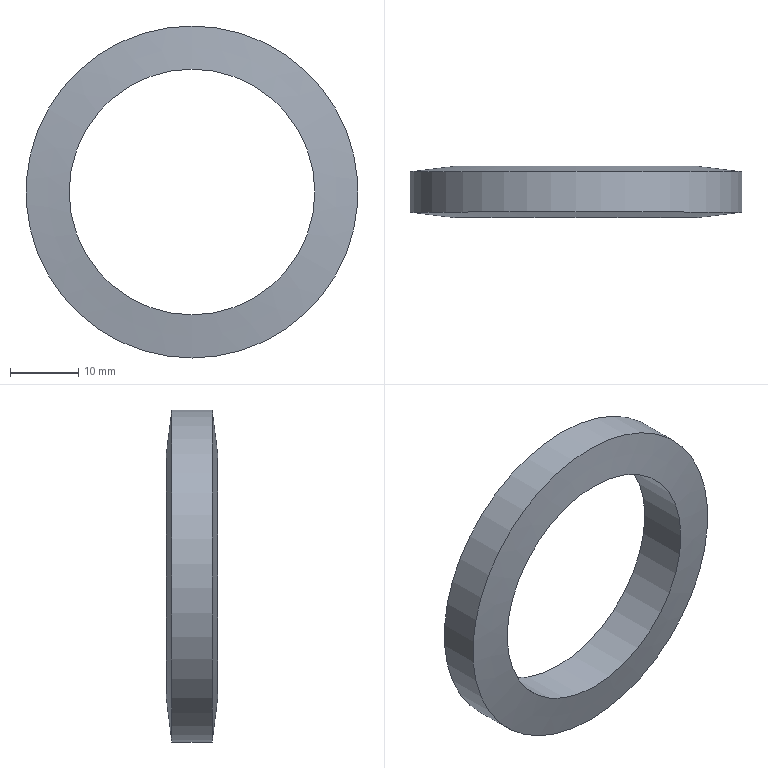Part | NX | features DATUM_CSYS 3, SKETCH 2, EXTRUDE 1, SWP104 1 | 1 solid | 4 faces | box 48.653 x 7.48 x 48.653 mm | volume 5606 mm3 | cone 2 | cylinder 2 | commonest cylinder face diameters 36 x1 48.653 x1
STEP:
#1=CARTESIAN_POINT('',(0.,-2.963,-24.327));
#2=VERTEX_POINT('',#1);
#3=CARTESIAN_POINT('',(0.,-2.963,0.));
#4=DIRECTION('',(0.,-1.,0.));
#5=DIRECTION('',(0.,0.,-1.));
#6=AXIS2_PLACEMENT_3D('',#3,#4,#5);
#7=CIRCLE('',#6,24.327);
#8=EDGE_CURVE('',#2,#2,#7,.T.);
#9=ORIENTED_EDGE('',*,*,#8,.T.);
#10=EDGE_LOOP('',(#9));
#11=FACE_BOUND('',#10,.T.);
#12=CARTESIAN_POINT('',(0.,-3.74,18.));
#13=VERTEX_POINT('',#12);
#14=CARTESIAN_POINT('',(0.,-3.74,0.));
#15=DIRECTION('',(0.,1.,0.));
#16=DIRECTION('',(0.,0.,1.));
#17=AXIS2_PLACEMENT_3D('',#14,#15,#16);
#18=CIRCLE('',#17,18.);
#19=EDGE_CURVE('',#13,#13,#18,.T.);
#20=ORIENTED_EDGE('',*,*,#19,.T.);
#21=EDGE_LOOP('',(#20));
#22=FACE_BOUND('',#21,.T.);
#23=CARTESIAN_POINT('',(0.,-5.95,0.));
#24=DIRECTION('',(0.,1.,0.));
#25=DIRECTION('',(0.,0.,1.));
#26=AXIS2_PLACEMENT_3D('',#23,#24,#25);
#27=CONICAL_SURFACE('',#26,0.,1.449);
#28=ADVANCED_FACE('',(#11,#22),#27,.T.);
#29=CARTESIAN_POINT('',(0.,2.963,-24.327));
#30=VERTEX_POINT('',#29);
#31=CARTESIAN_POINT('',(0.,2.963,0.));
#32=DIRECTION('',(0.,-1.,0.));
#33=DIRECTION('',(0.,0.,-1.));
#34=AXIS2_PLACEMENT_3D('',#31,#32,#33);
#35=CIRCLE('',#34,24.327);
#36=EDGE_CURVE('',#30,#30,#35,.T.);
#37=ORIENTED_EDGE('',*,*,#36,.F.);
#38=EDGE_LOOP('',(#37));
#39=FACE_BOUND('',#38,.T.);
#40=CARTESIAN_POINT('',(0.,3.74,-18.));
#41=VERTEX_POINT('',#40);
#42=CARTESIAN_POINT('',(0.,3.74,0.));
#43=DIRECTION('',(0.,-1.,0.));
#44=DIRECTION('',(0.,0.,-1.));
#45=AXIS2_PLACEMENT_3D('',#42,#43,#44);
#46=CIRCLE('',#45,18.);
#47=EDGE_CURVE('',#41,#41,#46,.T.);
#48=ORIENTED_EDGE('',*,*,#47,.T.);
#49=EDGE_LOOP('',(#48));
#50=FACE_BOUND('',#49,.T.);
#51=CARTESIAN_POINT('',(0.,2.963,0.));
#52=DIRECTION('',(0.,-1.,0.));
#53=DIRECTION('',(0.,0.,-1.));
#54=AXIS2_PLACEMENT_3D('',#51,#52,#53);
#55=CONICAL_SURFACE('',#54,24.327,1.449);
#56=ADVANCED_FACE('',(#39,#50),#55,.T.);
#57=ORIENTED_EDGE('',*,*,#36,.T.);
#58=EDGE_LOOP('',(#57));
#59=FACE_BOUND('',#58,.T.);
#60=ORIENTED_EDGE('',*,*,#8,.F.);
#61=EDGE_LOOP('',(#60));
#62=FACE_BOUND('',#61,.T.);
#63=CARTESIAN_POINT('',(0.,0.,0.));
#64=DIRECTION('',(0.,-1.,0.));
#65=DIRECTION('',(0.,0.,-1.));
#66=AXIS2_PLACEMENT_3D('',#63,#64,#65);
#67=CYLINDRICAL_SURFACE('',#66,24.327);
#68=ADVANCED_FACE('',(#59,#62),#67,.T.);
#69=ORIENTED_EDGE('',*,*,#19,.F.);
#70=EDGE_LOOP('',(#69));
#71=FACE_BOUND('',#70,.T.);
#72=ORIENTED_EDGE('',*,*,#47,.F.);
#73=EDGE_LOOP('',(#72));
#74=FACE_BOUND('',#73,.T.);
#75=CARTESIAN_POINT('',(0.,75.,0.));
#76=DIRECTION('',(0.,-1.,0.));
#77=DIRECTION('',(0.,0.,-1.));
#78=AXIS2_PLACEMENT_3D('',#75,#76,#77);
#79=CYLINDRICAL_SURFACE('',#78,18.);
#80=ADVANCED_FACE('',(#71,#74),#79,.F.);
#81=CLOSED_SHELL('',(#28,#56,#68,#80));
#82=MANIFOLD_SOLID_BREP('',#81);
#83=(LENGTH_UNIT()NAMED_UNIT(*)SI_UNIT(.MILLI.,.METRE.));
#84=UNCERTAINTY_MEASURE_WITH_UNIT(LENGTH_MEASURE(0.00001),#83,'','');
#85=(NAMED_UNIT(*)PLANE_ANGLE_UNIT()SI_UNIT($,.RADIAN.));
#86=(NAMED_UNIT(*)SI_UNIT($,.STERADIAN.)SOLID_ANGLE_UNIT());
#87=(GEOMETRIC_REPRESENTATION_CONTEXT(3)GLOBAL_UNCERTAINTY_ASSIGNED_CONTEXT((#84))GLOBAL_UNIT_ASSIGNED_CONTEXT((#83,#85,#86))REPRESENTATION_CONTEXT('',''));
#88=ADVANCED_BREP_SHAPE_REPRESENTATION('',(#82),#87);